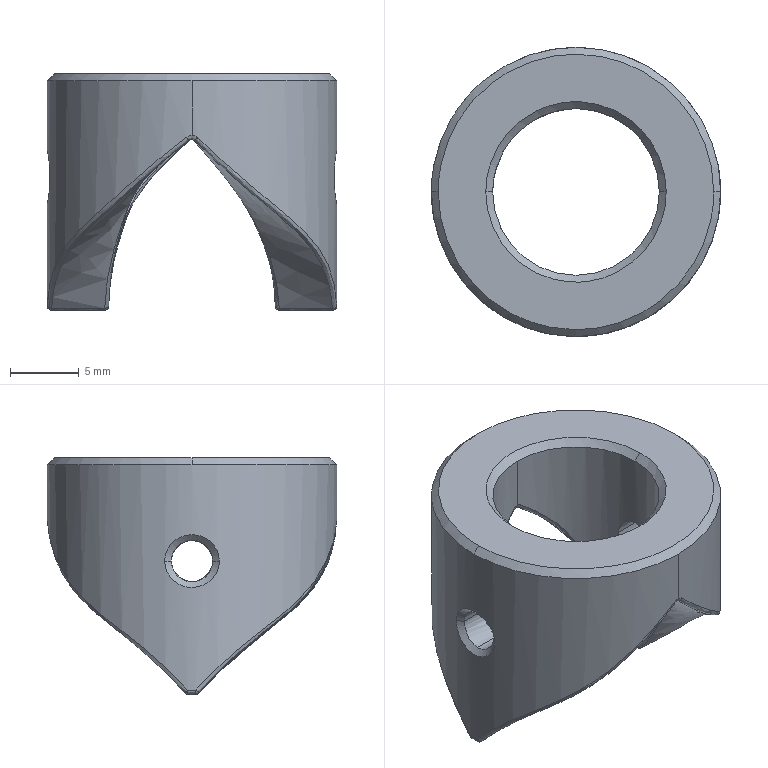Part | STEP file | 101000008264 | 1 solid | 60 faces | volume 2402 mm3 | spline 49 | cylinder 4 | cone 4 | plane 3 | commonest cylinder face diameters 12.1 x2 21 x2